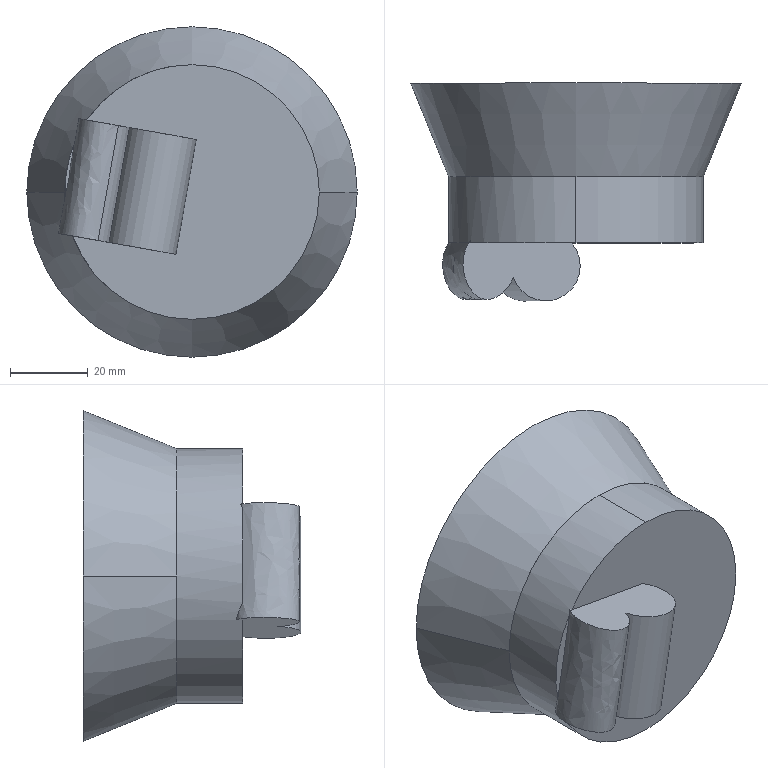Part | SolidWorks | features BaseBody 1 | 1 solid | 14 faces | box 85 x 56.019 x 85 mm | volume 176710 mm3 | plane 5 | cone 4 | cylinder 4 | spline 1 | commonest cylinder face diameters 18 x2 65.509 x2